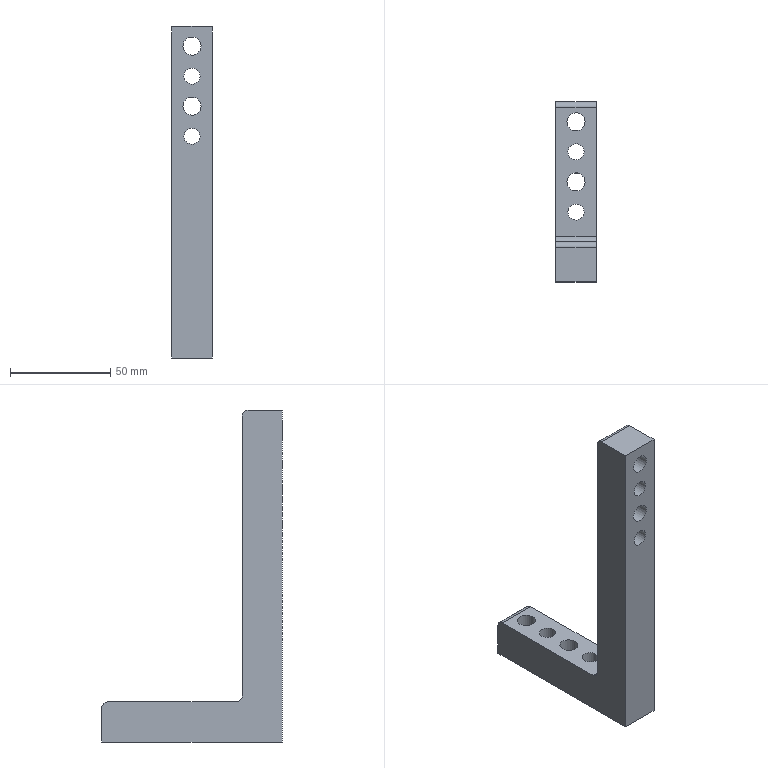Part | STEP file | SN10_008_003_SUPORTE | 1 solid | 19 faces | box 20 x 90 x 165.5 mm | volume 85051 mm3 | cylinder 11 | plane 8 | commonest cylinder face diameters 8 x4 9 x4 6 x3